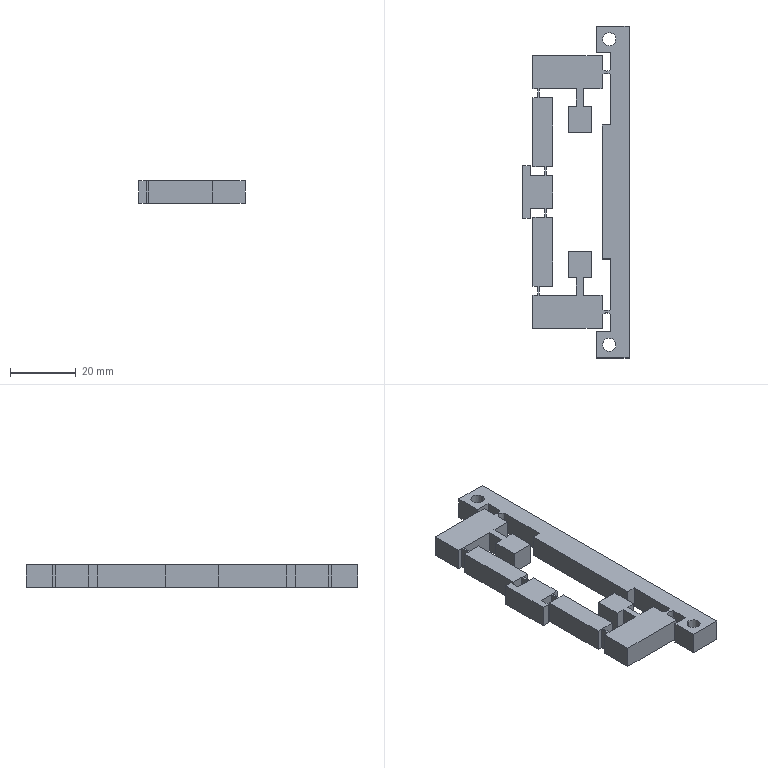Part | NX | features BREP 1 | 1 solid | 84 faces | box 32.2 x 100.6 x 6.8 mm | volume 11071 mm3 | plane 74 | cylinder 10 | commonest cylinder face diameters 4 x4 3.356 x3 3.36 x3